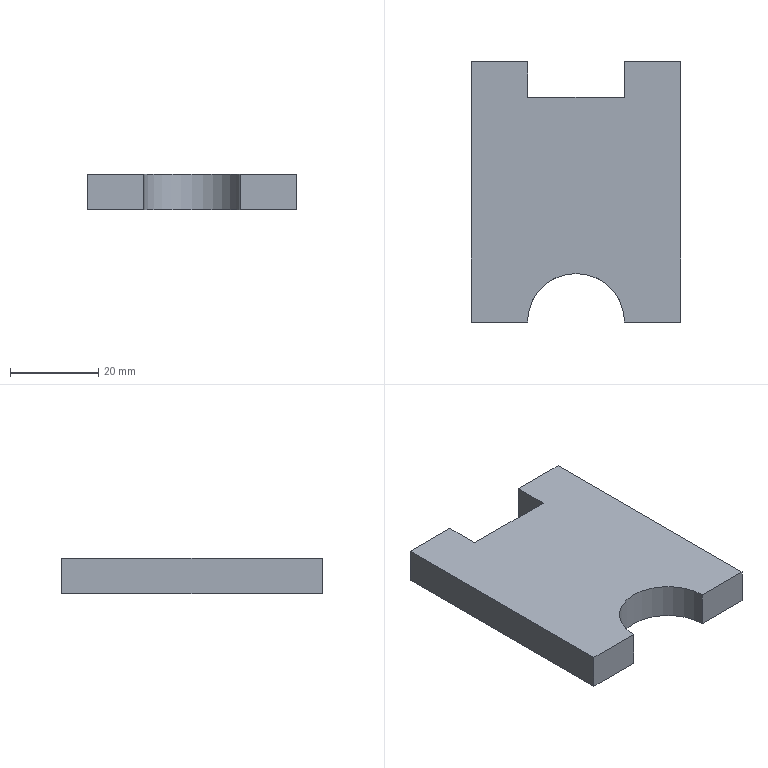Part | SolidWorks | features Extrusion 1 | 1 solid | 12 faces | box 47.495 x 59 x 8 mm | volume 19489 mm3 | plane 11 | cylinder 1 | commonest cylinder face diameters 22 x1
STEP:
#1=CARTESIAN_POINT('',(-229.288,91.149,0.));
#2=VERTEX_POINT('',#1);
#3=CARTESIAN_POINT('',(-229.288,99.149,0.));
#4=VERTEX_POINT('',#3);
#5=CARTESIAN_POINT('',(-229.288,99.149,0.));
#6=DIRECTION('',(0.,1.,0.));
#7=VECTOR('',#6,1000.);
#8=LINE('',#5,#7);
#9=EDGE_CURVE('',#2,#4,#8,.T.);
#10=ORIENTED_EDGE('',*,*,#9,.T.);
#11=CARTESIAN_POINT('',(-229.288,99.149,8.));
#12=VERTEX_POINT('',#11);
#13=CARTESIAN_POINT('',(-229.288,99.149,8.));
#14=DIRECTION('',(0.,0.,-1.));
#15=VECTOR('',#14,1000.);
#16=LINE('',#13,#15);
#17=EDGE_CURVE('',#12,#4,#16,.T.);
#18=ORIENTED_EDGE('',*,*,#17,.F.);
#19=CARTESIAN_POINT('',(-229.288,91.149,8.));
#20=VERTEX_POINT('',#19);
#21=CARTESIAN_POINT('',(-229.288,99.149,8.));
#22=DIRECTION('',(0.,1.,0.));
#23=VECTOR('',#22,1000.);
#24=LINE('',#21,#23);
#25=EDGE_CURVE('',#20,#12,#24,.T.);
#26=ORIENTED_EDGE('',*,*,#25,.F.);
#27=CARTESIAN_POINT('',(-229.288,91.149,8.));
#28=DIRECTION('',(0.,0.,-1.));
#29=VECTOR('',#28,1000.);
#30=LINE('',#27,#29);
#31=EDGE_CURVE('',#20,#2,#30,.T.);
#32=ORIENTED_EDGE('',*,*,#31,.T.);
#33=EDGE_LOOP('',(#10,#18,#26,#32));
#34=FACE_OUTER_BOUND('',#33,.T.);
#35=CARTESIAN_POINT('',(-229.288,99.149,8.));
#36=DIRECTION('',(-1.,0.,0.));
#37=DIRECTION('',(0.,-1.,0.));
#38=AXIS2_PLACEMENT_3D('',#35,#36,#37);
#39=PLANE('',#38);
#40=ADVANCED_FACE('',(#34),#39,.F.);
#41=CARTESIAN_POINT('',(-242.038,99.149,0.));
#42=VERTEX_POINT('',#41);
#43=CARTESIAN_POINT('',(-242.038,99.149,0.));
#44=DIRECTION('',(-1.,0.,0.));
#45=VECTOR('',#44,1000.);
#46=LINE('',#43,#45);
#47=EDGE_CURVE('',#4,#42,#46,.T.);
#48=ORIENTED_EDGE('',*,*,#47,.T.);
#49=CARTESIAN_POINT('',(-242.038,99.149,8.));
#50=VERTEX_POINT('',#49);
#51=CARTESIAN_POINT('',(-242.038,99.149,8.));
#52=DIRECTION('',(0.,0.,-1.));
#53=VECTOR('',#52,1000.);
#54=LINE('',#51,#53);
#55=EDGE_CURVE('',#50,#42,#54,.T.);
#56=ORIENTED_EDGE('',*,*,#55,.F.);
#57=CARTESIAN_POINT('',(-242.038,99.149,8.));
#58=DIRECTION('',(-1.,0.,0.));
#59=VECTOR('',#58,1000.);
#60=LINE('',#57,#59);
#61=EDGE_CURVE('',#12,#50,#60,.T.);
#62=ORIENTED_EDGE('',*,*,#61,.F.);
#63=ORIENTED_EDGE('',*,*,#17,.T.);
#64=EDGE_LOOP('',(#48,#56,#62,#63));
#65=FACE_OUTER_BOUND('',#64,.T.);
#66=CARTESIAN_POINT('',(-242.038,99.149,8.));
#67=DIRECTION('',(0.,-1.,0.));
#68=DIRECTION('',(1.,0.,0.));
#69=AXIS2_PLACEMENT_3D('',#66,#67,#68);
#70=PLANE('',#69);
#71=ADVANCED_FACE('',(#65),#70,.F.);
#72=CARTESIAN_POINT('',(-242.038,40.149,0.));
#73=VERTEX_POINT('',#72);
#74=CARTESIAN_POINT('',(-242.038,99.149,0.));
#75=DIRECTION('',(0.,-1.,0.));
#76=VECTOR('',#75,1000.);
#77=LINE('',#74,#76);
#78=EDGE_CURVE('',#42,#73,#77,.T.);
#79=ORIENTED_EDGE('',*,*,#78,.T.);
#80=CARTESIAN_POINT('',(-242.038,40.149,8.));
#81=VERTEX_POINT('',#80);
#82=CARTESIAN_POINT('',(-242.038,40.149,8.));
#83=DIRECTION('',(0.,0.,-1.));
#84=VECTOR('',#83,1000.);
#85=LINE('',#82,#84);
#86=EDGE_CURVE('',#81,#73,#85,.T.);
#87=ORIENTED_EDGE('',*,*,#86,.F.);
#88=CARTESIAN_POINT('',(-242.038,99.149,8.));
#89=DIRECTION('',(0.,-1.,0.));
#90=VECTOR('',#89,1000.);
#91=LINE('',#88,#90);
#92=EDGE_CURVE('',#50,#81,#91,.T.);
#93=ORIENTED_EDGE('',*,*,#92,.F.);
#94=ORIENTED_EDGE('',*,*,#55,.T.);
#95=EDGE_LOOP('',(#79,#87,#93,#94));
#96=FACE_OUTER_BOUND('',#95,.T.);
#97=CARTESIAN_POINT('',(-242.038,99.149,8.));
#98=DIRECTION('',(1.,0.,0.));
#99=DIRECTION('',(0.,1.,0.));
#100=AXIS2_PLACEMENT_3D('',#97,#98,#99);
#101=PLANE('',#100);
#102=ADVANCED_FACE('',(#96),#101,.F.);
#103=CARTESIAN_POINT('',(-229.29,40.149,0.));
#104=VERTEX_POINT('',#103);
#105=CARTESIAN_POINT('',(-242.038,40.149,0.));
#106=DIRECTION('',(1.,0.,0.));
#107=VECTOR('',#106,1000.);
#108=LINE('',#105,#107);
#109=EDGE_CURVE('',#73,#104,#108,.T.);
#110=ORIENTED_EDGE('',*,*,#109,.T.);
#111=CARTESIAN_POINT('',(-229.29,40.149,8.));
#112=VERTEX_POINT('',#111);
#113=CARTESIAN_POINT('',(-229.29,40.149,8.));
#114=DIRECTION('',(0.,0.,-1.));
#115=VECTOR('',#114,1000.);
#116=LINE('',#113,#115);
#117=EDGE_CURVE('',#112,#104,#116,.T.);
#118=ORIENTED_EDGE('',*,*,#117,.F.);
#119=CARTESIAN_POINT('',(-242.038,40.149,8.));
#120=DIRECTION('',(1.,0.,0.));
#121=VECTOR('',#120,1000.);
#122=LINE('',#119,#121);
#123=EDGE_CURVE('',#81,#112,#122,.T.);
#124=ORIENTED_EDGE('',*,*,#123,.F.);
#125=ORIENTED_EDGE('',*,*,#86,.T.);
#126=EDGE_LOOP('',(#110,#118,#124,#125));
#127=FACE_OUTER_BOUND('',#126,.T.);
#128=CARTESIAN_POINT('',(-242.038,40.149,8.));
#129=DIRECTION('',(0.,1.,0.));
#130=DIRECTION('',(-1.,0.,0.));
#131=AXIS2_PLACEMENT_3D('',#128,#129,#130);
#132=PLANE('',#131);
#133=ADVANCED_FACE('',(#127),#132,.F.);
#134=CARTESIAN_POINT('',(-207.29,40.149,0.));
#135=VERTEX_POINT('',#134);
#136=CARTESIAN_POINT('',(-218.29,40.149,0.));
#137=DIRECTION('',(0.,0.,-1.));
#138=DIRECTION('',(1.,0.,0.));
#139=AXIS2_PLACEMENT_3D('',#136,#137,#138);
#140=CIRCLE('',#139,11.);
#141=EDGE_CURVE('',#104,#135,#140,.T.);
#142=ORIENTED_EDGE('',*,*,#141,.T.);
#143=CARTESIAN_POINT('',(-207.29,40.149,8.));
#144=VERTEX_POINT('',#143);
#145=CARTESIAN_POINT('',(-207.29,40.149,8.));
#146=DIRECTION('',(0.,0.,-1.));
#147=VECTOR('',#146,1000.);
#148=LINE('',#145,#147);
#149=EDGE_CURVE('',#144,#135,#148,.T.);
#150=ORIENTED_EDGE('',*,*,#149,.F.);
#151=CARTESIAN_POINT('',(-218.29,40.149,8.));
#152=DIRECTION('',(0.,0.,-1.));
#153=DIRECTION('',(1.,0.,0.));
#154=AXIS2_PLACEMENT_3D('',#151,#152,#153);
#155=CIRCLE('',#154,11.);
#156=EDGE_CURVE('',#112,#144,#155,.T.);
#157=ORIENTED_EDGE('',*,*,#156,.F.);
#158=ORIENTED_EDGE('',*,*,#117,.T.);
#159=EDGE_LOOP('',(#142,#150,#157,#158));
#160=FACE_OUTER_BOUND('',#159,.T.);
#161=CARTESIAN_POINT('',(-218.29,40.149,8.));
#162=DIRECTION('',(0.,0.,-1.));
#163=DIRECTION('',(-1.,0.,0.));
#164=AXIS2_PLACEMENT_3D('',#161,#162,#163);
#165=CYLINDRICAL_SURFACE('',#164,11.);
#166=ADVANCED_FACE('',(#160),#165,.F.);
#167=CARTESIAN_POINT('',(-194.543,40.149,0.));
#168=VERTEX_POINT('',#167);
#169=CARTESIAN_POINT('',(-194.543,40.149,0.));
#170=DIRECTION('',(1.,0.,0.));
#171=VECTOR('',#170,1000.);
#172=LINE('',#169,#171);
#173=EDGE_CURVE('',#135,#168,#172,.T.);
#174=ORIENTED_EDGE('',*,*,#173,.T.);
#175=CARTESIAN_POINT('',(-194.543,40.149,8.));
#176=VERTEX_POINT('',#175);
#177=CARTESIAN_POINT('',(-194.543,40.149,8.));
#178=DIRECTION('',(0.,0.,-1.));
#179=VECTOR('',#178,1000.);
#180=LINE('',#177,#179);
#181=EDGE_CURVE('',#176,#168,#180,.T.);
#182=ORIENTED_EDGE('',*,*,#181,.F.);
#183=CARTESIAN_POINT('',(-194.543,40.149,8.));
#184=DIRECTION('',(1.,0.,0.));
#185=VECTOR('',#184,1000.);
#186=LINE('',#183,#185);
#187=EDGE_CURVE('',#144,#176,#186,.T.);
#188=ORIENTED_EDGE('',*,*,#187,.F.);
#189=ORIENTED_EDGE('',*,*,#149,.T.);
#190=EDGE_LOOP('',(#174,#182,#188,#189));
#191=FACE_OUTER_BOUND('',#190,.T.);
#192=CARTESIAN_POINT('',(-194.543,40.149,8.));
#193=DIRECTION('',(0.,1.,0.));
#194=DIRECTION('',(-1.,0.,0.));
#195=AXIS2_PLACEMENT_3D('',#192,#193,#194);
#196=PLANE('',#195);
#197=ADVANCED_FACE('',(#191),#196,.F.);
#198=CARTESIAN_POINT('',(-194.543,99.149,0.));
#199=VERTEX_POINT('',#198);
#200=CARTESIAN_POINT('',(-194.543,40.149,0.));
#201=DIRECTION('',(0.,1.,0.));
#202=VECTOR('',#201,1000.);
#203=LINE('',#200,#202);
#204=EDGE_CURVE('',#168,#199,#203,.T.);
#205=ORIENTED_EDGE('',*,*,#204,.T.);
#206=CARTESIAN_POINT('',(-194.543,99.149,8.));
#207=VERTEX_POINT('',#206);
#208=CARTESIAN_POINT('',(-194.543,99.149,8.));
#209=DIRECTION('',(0.,0.,-1.));
#210=VECTOR('',#209,1000.);
#211=LINE('',#208,#210);
#212=EDGE_CURVE('',#207,#199,#211,.T.);
#213=ORIENTED_EDGE('',*,*,#212,.F.);
#214=CARTESIAN_POINT('',(-194.543,40.149,8.));
#215=DIRECTION('',(0.,1.,0.));
#216=VECTOR('',#215,1000.);
#217=LINE('',#214,#216);
#218=EDGE_CURVE('',#176,#207,#217,.T.);
#219=ORIENTED_EDGE('',*,*,#218,.F.);
#220=ORIENTED_EDGE('',*,*,#181,.T.);
#221=EDGE_LOOP('',(#205,#213,#219,#220));
#222=FACE_OUTER_BOUND('',#221,.T.);
#223=CARTESIAN_POINT('',(-194.543,40.149,8.));
#224=DIRECTION('',(-1.,0.,0.));
#225=DIRECTION('',(0.,0.,1.));
#226=AXIS2_PLACEMENT_3D('',#223,#224,#225);
#227=PLANE('',#226);
#228=ADVANCED_FACE('',(#222),#227,.F.);
#229=CARTESIAN_POINT('',(-207.288,99.149,0.));
#230=VERTEX_POINT('',#229);
#231=CARTESIAN_POINT('',(-194.543,99.149,0.));
#232=DIRECTION('',(-1.,0.,0.));
#233=VECTOR('',#232,1000.);
#234=LINE('',#231,#233);
#235=EDGE_CURVE('',#199,#230,#234,.T.);
#236=ORIENTED_EDGE('',*,*,#235,.T.);
#237=CARTESIAN_POINT('',(-207.288,99.149,8.));
#238=VERTEX_POINT('',#237);
#239=CARTESIAN_POINT('',(-207.288,99.149,8.));
#240=DIRECTION('',(0.,0.,-1.));
#241=VECTOR('',#240,1000.);
#242=LINE('',#239,#241);
#243=EDGE_CURVE('',#238,#230,#242,.T.);
#244=ORIENTED_EDGE('',*,*,#243,.F.);
#245=CARTESIAN_POINT('',(-194.543,99.149,8.));
#246=DIRECTION('',(-1.,0.,0.));
#247=VECTOR('',#246,1000.);
#248=LINE('',#245,#247);
#249=EDGE_CURVE('',#207,#238,#248,.T.);
#250=ORIENTED_EDGE('',*,*,#249,.F.);
#251=ORIENTED_EDGE('',*,*,#212,.T.);
#252=EDGE_LOOP('',(#236,#244,#250,#251));
#253=FACE_OUTER_BOUND('',#252,.T.);
#254=CARTESIAN_POINT('',(-194.543,99.149,8.));
#255=DIRECTION('',(0.,-1.,0.));
#256=DIRECTION('',(0.,0.,-1.));
#257=AXIS2_PLACEMENT_3D('',#254,#255,#256);
#258=PLANE('',#257);
#259=ADVANCED_FACE('',(#253),#258,.F.);
#260=CARTESIAN_POINT('',(-207.288,91.149,0.));
#261=VERTEX_POINT('',#260);
#262=CARTESIAN_POINT('',(-207.288,99.149,0.));
#263=DIRECTION('',(0.,-1.,0.));
#264=VECTOR('',#263,1000.);
#265=LINE('',#262,#264);
#266=EDGE_CURVE('',#230,#261,#265,.T.);
#267=ORIENTED_EDGE('',*,*,#266,.T.);
#268=CARTESIAN_POINT('',(-207.288,91.149,8.));
#269=VERTEX_POINT('',#268);
#270=CARTESIAN_POINT('',(-207.288,91.149,8.));
#271=DIRECTION('',(0.,0.,-1.));
#272=VECTOR('',#271,1000.);
#273=LINE('',#270,#272);
#274=EDGE_CURVE('',#269,#261,#273,.T.);
#275=ORIENTED_EDGE('',*,*,#274,.F.);
#276=CARTESIAN_POINT('',(-207.288,99.149,8.));
#277=DIRECTION('',(0.,-1.,0.));
#278=VECTOR('',#277,1000.);
#279=LINE('',#276,#278);
#280=EDGE_CURVE('',#238,#269,#279,.T.);
#281=ORIENTED_EDGE('',*,*,#280,.F.);
#282=ORIENTED_EDGE('',*,*,#243,.T.);
#283=EDGE_LOOP('',(#267,#275,#281,#282));
#284=FACE_OUTER_BOUND('',#283,.T.);
#285=CARTESIAN_POINT('',(-207.288,99.149,8.));
#286=DIRECTION('',(1.,0.,0.));
#287=DIRECTION('',(0.,1.,0.));
#288=AXIS2_PLACEMENT_3D('',#285,#286,#287);
#289=PLANE('',#288);
#290=ADVANCED_FACE('',(#284),#289,.F.);
#291=CARTESIAN_POINT('',(-229.288,91.149,0.));
#292=DIRECTION('',(-1.,0.,0.));
#293=VECTOR('',#292,1000.);
#294=LINE('',#291,#293);
#295=EDGE_CURVE('',#261,#2,#294,.T.);
#296=ORIENTED_EDGE('',*,*,#295,.T.);
#297=ORIENTED_EDGE('',*,*,#31,.F.);
#298=CARTESIAN_POINT('',(-229.288,91.149,8.));
#299=DIRECTION('',(-1.,0.,0.));
#300=VECTOR('',#299,1000.);
#301=LINE('',#298,#300);
#302=EDGE_CURVE('',#269,#20,#301,.T.);
#303=ORIENTED_EDGE('',*,*,#302,.F.);
#304=ORIENTED_EDGE('',*,*,#274,.T.);
#305=EDGE_LOOP('',(#296,#297,#303,#304));
#306=FACE_OUTER_BOUND('',#305,.T.);
#307=CARTESIAN_POINT('',(-229.288,91.149,8.));
#308=DIRECTION('',(0.,-1.,0.));
#309=DIRECTION('',(1.,0.,0.));
#310=AXIS2_PLACEMENT_3D('',#307,#308,#309);
#311=PLANE('',#310);
#312=ADVANCED_FACE('',(#306),#311,.F.);
#313=ORIENTED_EDGE('',*,*,#25,.T.);
#314=ORIENTED_EDGE('',*,*,#61,.T.);
#315=ORIENTED_EDGE('',*,*,#92,.T.);
#316=ORIENTED_EDGE('',*,*,#123,.T.);
#317=ORIENTED_EDGE('',*,*,#156,.T.);
#318=ORIENTED_EDGE('',*,*,#187,.T.);
#319=ORIENTED_EDGE('',*,*,#218,.T.);
#320=ORIENTED_EDGE('',*,*,#249,.T.);
#321=ORIENTED_EDGE('',*,*,#280,.T.);
#322=ORIENTED_EDGE('',*,*,#302,.T.);
#323=EDGE_LOOP('',(#313,#314,#315,#316,#317,#318,#319,#320,#321,#322));
#324=FACE_OUTER_BOUND('',#323,.T.);
#325=CARTESIAN_POINT('',(-218.29,40.149,8.));
#326=DIRECTION('',(0.,0.,1.));
#327=DIRECTION('',(1.,0.,0.));
#328=AXIS2_PLACEMENT_3D('',#325,#326,#327);
#329=PLANE('',#328);
#330=ADVANCED_FACE('',(#324),#329,.T.);
#331=ORIENTED_EDGE('',*,*,#9,.F.);
#332=ORIENTED_EDGE('',*,*,#295,.F.);
#333=ORIENTED_EDGE('',*,*,#266,.F.);
#334=ORIENTED_EDGE('',*,*,#235,.F.);
#335=ORIENTED_EDGE('',*,*,#204,.F.);
#336=ORIENTED_EDGE('',*,*,#173,.F.);
#337=ORIENTED_EDGE('',*,*,#141,.F.);
#338=ORIENTED_EDGE('',*,*,#109,.F.);
#339=ORIENTED_EDGE('',*,*,#78,.F.);
#340=ORIENTED_EDGE('',*,*,#47,.F.);
#341=EDGE_LOOP('',(#331,#332,#333,#334,#335,#336,#337,#338,#339,#340));
#342=FACE_OUTER_BOUND('',#341,.T.);
#343=CARTESIAN_POINT('',(-218.29,40.149,0.));
#344=DIRECTION('',(0.,0.,1.));
#345=DIRECTION('',(1.,0.,0.));
#346=AXIS2_PLACEMENT_3D('',#343,#344,#345);
#347=PLANE('',#346);
#348=ADVANCED_FACE('',(#342),#347,.F.);
#349=CLOSED_SHELL('',(#40,#71,#102,#133,#166,#197,#228,#259,#290,#312,#330,#348));
#350=MANIFOLD_SOLID_BREP('',#349);
#351=CARTESIAN_POINT('',(0.,0.,0.));
#352=DIRECTION('',(0.,0.,1.));
#353=DIRECTION('',(1.,0.,0.));
#354=AXIS2_PLACEMENT_3D('',#351,#352,#353);
#355=(LENGTH_UNIT()NAMED_UNIT(*)SI_UNIT(.MILLI.,.METRE.));
#356=UNCERTAINTY_MEASURE_WITH_UNIT(LENGTH_MEASURE(0.00001),#355,'','');
#357=(NAMED_UNIT(*)PLANE_ANGLE_UNIT()SI_UNIT($,.RADIAN.));
#358=(NAMED_UNIT(*)SI_UNIT($,.STERADIAN.)SOLID_ANGLE_UNIT());
#359=(GEOMETRIC_REPRESENTATION_CONTEXT(3)GLOBAL_UNCERTAINTY_ASSIGNED_CONTEXT((#356))GLOBAL_UNIT_ASSIGNED_CONTEXT((#355,#357,#358))REPRESENTATION_CONTEXT('',''));
#360=ADVANCED_BREP_SHAPE_REPRESENTATION('',(#350,#354),#359);